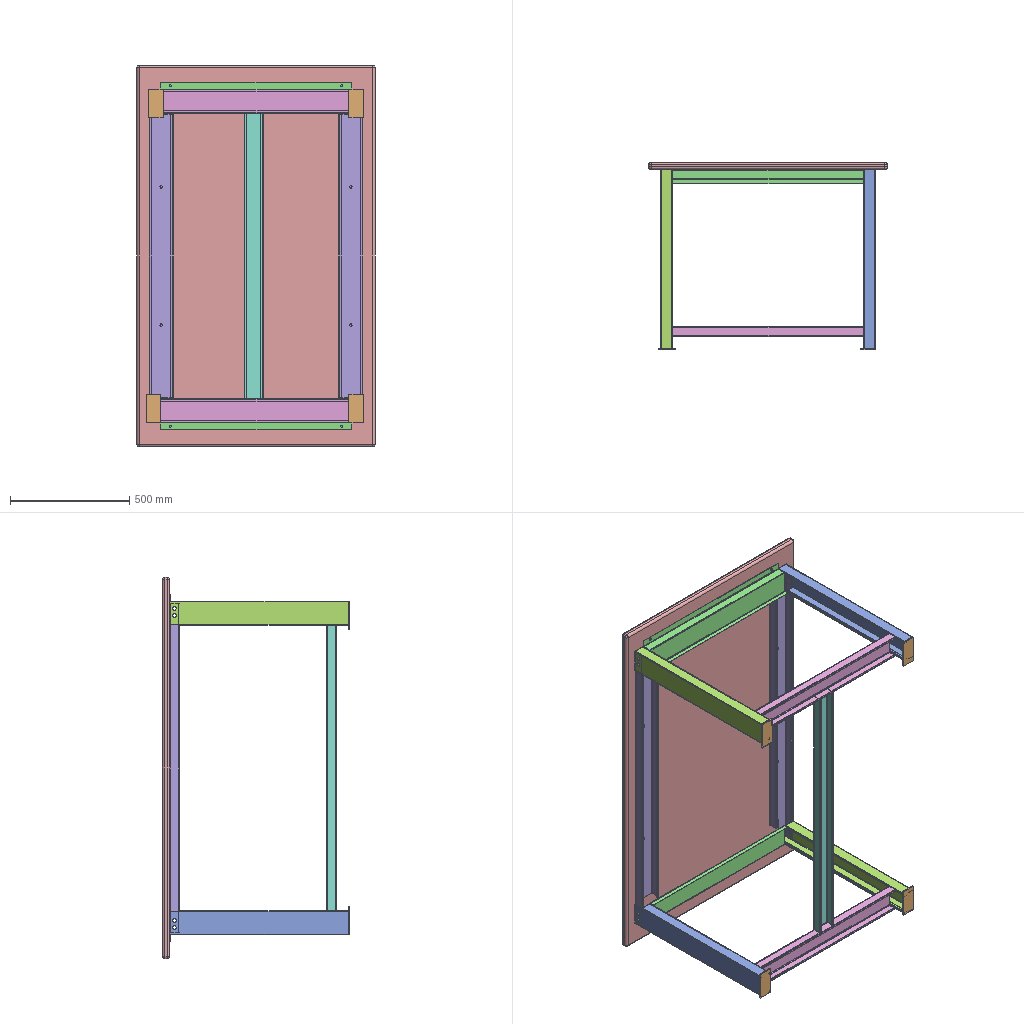Assembly | SolidWorks | 9 different items | 17 placed | box 1000 x 785 x 1600 mm
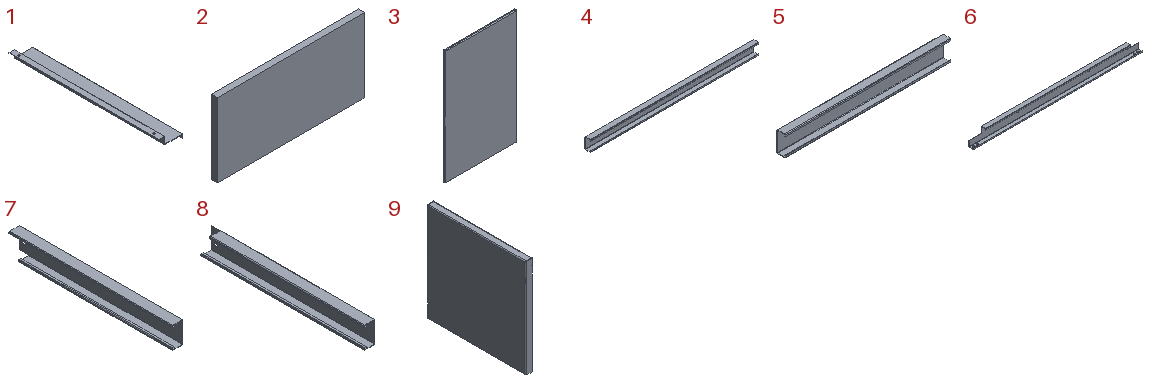Parts list (item | quantity | size | volume | features):
1 | x2 | 128 x 800 x 58 mm | 290508 mm3 | features EdgeFlange 3, FlatPattern 1, ICE 1, SMBaseFlange 1, SheetMetal 1
2 | x4 | 120 x 5 x 60 mm | 36000 mm3 | features Extrusion 1
3 | x1 | 1000 x 30 x 1600 mm | 47775578 mm3 | features Extrusion 1, Fillet 1
4 | x1 | 1200 x 40 x 80 mm | 402499 mm3 | features EdgeFlange 2, FlatPattern 1, SMBaseFlange 1, SheetMetal 1
5 | x2 | 800 x 40 x 100 mm | 300333 mm3 | features EdgeFlange 2, FlatPattern 1, SMBaseFlange 1, SheetMetal 1
6 | x2 | 1380 x 40 x 100 mm | 478771 mm3 | features EdgeFlange 2, ICE 2, FlatPattern 1, SMBaseFlange 1, SheetMetal 1
7 | x2 | 50 x 750 x 100 mm | 328411 mm3 | features EdgeFlange 3, ICE 2, FlatPattern 1, SMBaseFlange 1, SheetMetal 1
8 | x2 | 50 x 750 x 100 mm | 328548 mm3 | features EdgeFlange 3, ICE 3, FlatPattern 1, SMBaseFlange 1, SheetMetal 1
9 | x1 | 20 x 300 x 300 mm | 178165 mm3 | features EdgeFlange 3, CornerFeat 1, FlatPattern 1, SMBaseFlange 1, SheetMetal 1
Mates (type | each side: item.copy, entity, surface, feature):
Coincident | 3.1 face plane Boss-Extrude1 | 7.1 face plane Edge-Flange1
DistanceDim | 7.1 face plane Base-Flange1 | 3.1 face plane Boss-Extrude1
DistanceDim | 7.1 face plane Edge-Flange1 | 3.1 face plane Boss-Extrude1
Coincident | 3.1 face plane Boss-Extrude1 | 8.1 face plane Edge-Flange2
DistanceDim | 8.1 face plane Base-Flange1 | 3.1 face plane Boss-Extrude1
DistanceDim | 8.1 face plane Edge-Flange1 | 3.1 face plane Boss-Extrude1
Coincident | 3.1 face plane Boss-Extrude1 | 7.2 face plane Base-Flange1
DistanceDim | 7.2 face plane Base-Flange1 | 3.1 face plane Boss-Extrude1
DistanceDim | 7.2 face plane Edge-Flange1 | 3.1 face plane Boss-Extrude1
Coincident | 3.1 face plane Boss-Extrude1 | 8.2 face plane Edge-Flange1
Coincident | 7.2 face plane Base-Flange1 | 8.2 face plane Base-Flange1
DistanceDim | 8.2 face plane Edge-Flange1 | 3.1 face plane Boss-Extrude1
Coincident | 8.1 face plane Edge-Flange2 | 5.1 face plane Base-Flange1
Coincident | 8.1 face plane Edge-Flange1 | 5.1 face plane Edge-Flange1
DistanceDim | 8.1 face plane Edge-Flange3 | 5.1 face plane Edge-Flange2
Coincident | 7.1 face plane Edge-Flange1 | 5.2 face plane Edge-Flange1
Coincident | 7.1 face plane Edge-Flange2 | 5.2 face plane Base-Flange1
DistanceDim | 5.2 face plane Edge-Flange2 | 7.1 face plane Edge-Flange1
Coincident | 5.1 face plane Base-Flange1 | 4.1 face plane Base-Flange1
Coincident | 5.1 face plane Edge-Flange1 | 4.1 face plane Edge-Flange1
DistanceDim | 4.1 face plane Edge-Flange1 | 7.2 face plane Base-Flange1
Coincident | 8.1 face plane Edge bend 3 | 2.1 face plane Boss-Extrude1
Coincident | 8.1 face plane Base-Flange1 | 2.1 face plane Boss-Extrude1
Coincident | 8.1 face plane Edge-Flange1 | 2.1 face plane Boss-Extrude1
Coincident | 7.2 face plane Edge-Flange1 | 2.2 face plane Boss-Extrude1
Coincident | 7.2 face plane Base-Flange1 | 2.2 face plane Boss-Extrude1
Coincident | 7.2 face plane Edge-Flange2 | 2.2 face plane Boss-Extrude1
Coincident | 7.1 face plane Edge-Flange1 | 2.3 face plane Boss-Extrude1 | 2 times
Coincident | 7.1 face plane Base-Flange1 | 2.3 face plane Boss-Extrude1
Coincident | 8.2 face plane Edge-Flange1 | 2.4 face plane Boss-Extrude1 | 2 times
Coincident | 8.2 face plane Base-Flange1 | 2.4 face plane Boss-Extrude1
Coincident | 3.1 face plane Boss-Extrude1 | 6.1 face plane Base-Flange1
Coincident | 7.1 face plane Edge-Flange3 | 6.1 face plane Base-Flange1
Coincident | 7.1 face plane Base-Flange1 | 6.1 face plane Edge-Flange1
Coincident | 3.1 face plane Boss-Extrude1 | 6.2 face plane Base-Flange1
Coincident | 7.2 face plane Base-Flange1 | 6.2 face plane Edge-Flange1
Coincident | 7.2 face plane Edge-Flange3 | 6.2 face plane Edge bend 2
Coincident | 3.1 face plane Boss-Extrude1 | 1.1 face plane Edge-Flange3
Coincident | 6.1 face plane Cut-Extrude2 | 1.1 face plane Edge-Flange1
Coincident | 7.1 face plane Edge-Flange1 | 1.1 face plane Edge-Flange1
Coincident | 3.1 face plane Boss-Extrude1 | 1.2 face plane Edge-Flange3
Coincident | 6.1 face plane Cut-Extrude2 | 1.2 face plane Edge-Flange1
Coincident | 8.1 face plane Edge-Flange1 | 1.2 face plane Edge-Flange1